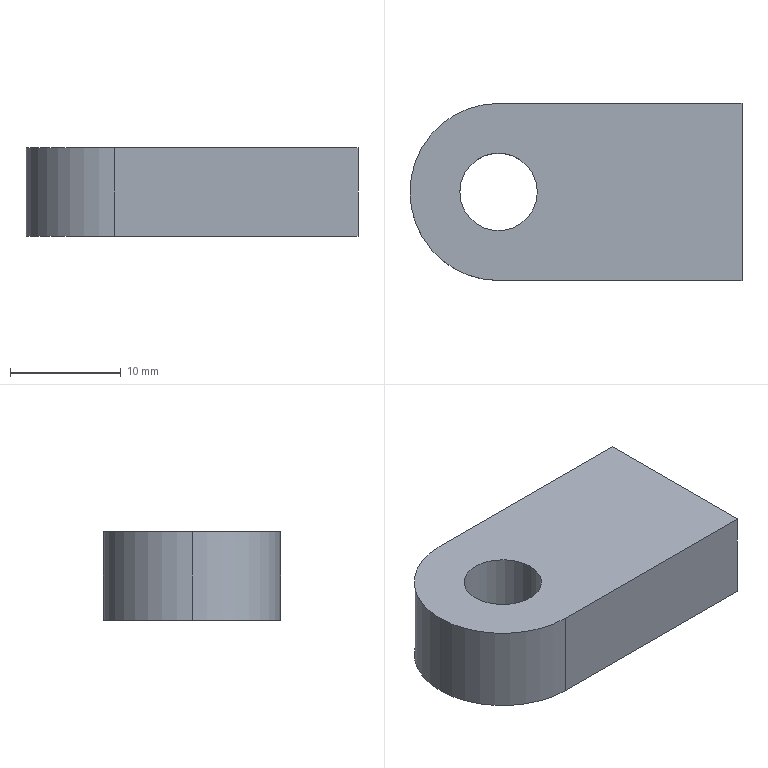Part | SolidWorks | features Extrusion 1 | 1 solid | 9 faces | box 30 x 16 x 8 mm | volume 3312 mm3 | plane 5 | cylinder 4 | commonest cylinder face diameters 7 x2 16 x2
STEP:
#1=CARTESIAN_POINT('',(-3.5,0.,8.));
#2=VERTEX_POINT('',#1);
#3=CARTESIAN_POINT('',(3.5,0.,8.));
#4=VERTEX_POINT('',#3);
#5=CARTESIAN_POINT('',(0.,0.,8.));
#6=DIRECTION('',(0.,0.,1.));
#7=DIRECTION('',(1.,0.,0.));
#8=AXIS2_PLACEMENT_3D('',#5,#6,#7);
#9=CIRCLE('',#8,3.5);
#10=EDGE_CURVE('',#2,#4,#9,.T.);
#11=ORIENTED_EDGE('',*,*,#10,.T.);
#12=CARTESIAN_POINT('',(3.5,0.,0.));
#13=VERTEX_POINT('',#12);
#14=CARTESIAN_POINT('',(3.5,0.,8.));
#15=DIRECTION('',(0.,0.,-1.));
#16=VECTOR('',#15,1000.);
#17=LINE('',#14,#16);
#18=EDGE_CURVE('',#4,#13,#17,.T.);
#19=ORIENTED_EDGE('',*,*,#18,.T.);
#20=CARTESIAN_POINT('',(-3.5,0.,0.));
#21=VERTEX_POINT('',#20);
#22=CARTESIAN_POINT('',(0.,0.,0.));
#23=DIRECTION('',(0.,0.,1.));
#24=DIRECTION('',(1.,0.,0.));
#25=AXIS2_PLACEMENT_3D('',#22,#23,#24);
#26=CIRCLE('',#25,3.5);
#27=EDGE_CURVE('',#21,#13,#26,.T.);
#28=ORIENTED_EDGE('',*,*,#27,.F.);
#29=CARTESIAN_POINT('',(-3.5,0.,8.));
#30=DIRECTION('',(0.,0.,-1.));
#31=VECTOR('',#30,1000.);
#32=LINE('',#29,#31);
#33=EDGE_CURVE('',#2,#21,#32,.T.);
#34=ORIENTED_EDGE('',*,*,#33,.F.);
#35=EDGE_LOOP('',(#11,#19,#28,#34));
#36=FACE_OUTER_BOUND('',#35,.T.);
#37=CARTESIAN_POINT('',(0.,0.,8.));
#38=DIRECTION('',(0.,0.,-1.));
#39=DIRECTION('',(-1.,0.,0.));
#40=AXIS2_PLACEMENT_3D('',#37,#38,#39);
#41=CYLINDRICAL_SURFACE('',#40,3.5);
#42=ADVANCED_FACE('',(#36),#41,.F.);
#43=CARTESIAN_POINT('',(-8.,0.,8.));
#44=VERTEX_POINT('',#43);
#45=CARTESIAN_POINT('',(0.,-8.,8.));
#46=VERTEX_POINT('',#45);
#47=CARTESIAN_POINT('',(0.,0.,8.));
#48=DIRECTION('',(0.,0.,1.));
#49=DIRECTION('',(1.,0.,0.));
#50=AXIS2_PLACEMENT_3D('',#47,#48,#49);
#51=CIRCLE('',#50,8.);
#52=EDGE_CURVE('',#44,#46,#51,.T.);
#53=ORIENTED_EDGE('',*,*,#52,.F.);
#54=CARTESIAN_POINT('',(-8.,0.,0.));
#55=VERTEX_POINT('',#54);
#56=CARTESIAN_POINT('',(-8.,0.,8.));
#57=DIRECTION('',(0.,0.,-1.));
#58=VECTOR('',#57,1000.);
#59=LINE('',#56,#58);
#60=EDGE_CURVE('',#44,#55,#59,.T.);
#61=ORIENTED_EDGE('',*,*,#60,.T.);
#62=CARTESIAN_POINT('',(0.,-8.,0.));
#63=VERTEX_POINT('',#62);
#64=CARTESIAN_POINT('',(0.,0.,0.));
#65=DIRECTION('',(0.,0.,1.));
#66=DIRECTION('',(1.,0.,0.));
#67=AXIS2_PLACEMENT_3D('',#64,#65,#66);
#68=CIRCLE('',#67,8.);
#69=EDGE_CURVE('',#55,#63,#68,.T.);
#70=ORIENTED_EDGE('',*,*,#69,.T.);
#71=CARTESIAN_POINT('',(0.,-8.,8.));
#72=DIRECTION('',(0.,0.,-1.));
#73=VECTOR('',#72,1000.);
#74=LINE('',#71,#73);
#75=EDGE_CURVE('',#46,#63,#74,.T.);
#76=ORIENTED_EDGE('',*,*,#75,.F.);
#77=EDGE_LOOP('',(#53,#61,#70,#76));
#78=FACE_OUTER_BOUND('',#77,.T.);
#79=CARTESIAN_POINT('',(0.,0.,8.));
#80=DIRECTION('',(0.,0.,-1.));
#81=DIRECTION('',(-1.,0.,0.));
#82=AXIS2_PLACEMENT_3D('',#79,#80,#81);
#83=CYLINDRICAL_SURFACE('',#82,8.);
#84=ADVANCED_FACE('',(#78),#83,.T.);
#85=CARTESIAN_POINT('',(0.,8.,8.));
#86=VERTEX_POINT('',#85);
#87=CARTESIAN_POINT('',(0.,0.,8.));
#88=DIRECTION('',(0.,0.,1.));
#89=DIRECTION('',(1.,0.,0.));
#90=AXIS2_PLACEMENT_3D('',#87,#88,#89);
#91=CIRCLE('',#90,8.);
#92=EDGE_CURVE('',#86,#44,#91,.T.);
#93=ORIENTED_EDGE('',*,*,#92,.T.);
#94=ORIENTED_EDGE('',*,*,#52,.T.);
#95=CARTESIAN_POINT('',(22.,-8.,8.));
#96=VERTEX_POINT('',#95);
#97=CARTESIAN_POINT('',(22.,-8.,8.));
#98=DIRECTION('',(1.,0.,0.));
#99=VECTOR('',#98,1000.);
#100=LINE('',#97,#99);
#101=EDGE_CURVE('',#46,#96,#100,.T.);
#102=ORIENTED_EDGE('',*,*,#101,.T.);
#103=CARTESIAN_POINT('',(22.,8.,8.));
#104=VERTEX_POINT('',#103);
#105=CARTESIAN_POINT('',(22.,8.,8.));
#106=DIRECTION('',(0.,1.,0.));
#107=VECTOR('',#106,1000.);
#108=LINE('',#105,#107);
#109=EDGE_CURVE('',#96,#104,#108,.T.);
#110=ORIENTED_EDGE('',*,*,#109,.T.);
#111=CARTESIAN_POINT('',(0.,8.,8.));
#112=DIRECTION('',(-1.,0.,0.));
#113=VECTOR('',#112,1000.);
#114=LINE('',#111,#113);
#115=EDGE_CURVE('',#104,#86,#114,.T.);
#116=ORIENTED_EDGE('',*,*,#115,.T.);
#117=EDGE_LOOP('',(#93,#94,#102,#110,#116));
#118=FACE_OUTER_BOUND('',#117,.T.);
#119=ORIENTED_EDGE('',*,*,#10,.F.);
#120=CARTESIAN_POINT('',(0.,0.,8.));
#121=DIRECTION('',(0.,0.,1.));
#122=DIRECTION('',(1.,0.,0.));
#123=AXIS2_PLACEMENT_3D('',#120,#121,#122);
#124=CIRCLE('',#123,3.5);
#125=EDGE_CURVE('',#4,#2,#124,.T.);
#126=ORIENTED_EDGE('',*,*,#125,.F.);
#127=EDGE_LOOP('',(#119,#126));
#128=FACE_BOUND('',#127,.T.);
#129=CARTESIAN_POINT('',(0.,0.,8.));
#130=DIRECTION('',(0.,0.,1.));
#131=DIRECTION('',(1.,0.,0.));
#132=AXIS2_PLACEMENT_3D('',#129,#130,#131);
#133=PLANE('',#132);
#134=ADVANCED_FACE('',(#118,#128),#133,.T.);
#135=CARTESIAN_POINT('',(0.,8.,0.));
#136=VERTEX_POINT('',#135);
#137=CARTESIAN_POINT('',(0.,0.,0.));
#138=DIRECTION('',(0.,0.,1.));
#139=DIRECTION('',(1.,0.,0.));
#140=AXIS2_PLACEMENT_3D('',#137,#138,#139);
#141=CIRCLE('',#140,8.);
#142=EDGE_CURVE('',#136,#55,#141,.T.);
#143=ORIENTED_EDGE('',*,*,#142,.F.);
#144=CARTESIAN_POINT('',(22.,8.,0.));
#145=VERTEX_POINT('',#144);
#146=CARTESIAN_POINT('',(0.,8.,0.));
#147=DIRECTION('',(-1.,0.,0.));
#148=VECTOR('',#147,1000.);
#149=LINE('',#146,#148);
#150=EDGE_CURVE('',#145,#136,#149,.T.);
#151=ORIENTED_EDGE('',*,*,#150,.F.);
#152=CARTESIAN_POINT('',(22.,-8.,0.));
#153=VERTEX_POINT('',#152);
#154=CARTESIAN_POINT('',(22.,8.,0.));
#155=DIRECTION('',(0.,1.,0.));
#156=VECTOR('',#155,1000.);
#157=LINE('',#154,#156);
#158=EDGE_CURVE('',#153,#145,#157,.T.);
#159=ORIENTED_EDGE('',*,*,#158,.F.);
#160=CARTESIAN_POINT('',(22.,-8.,0.));
#161=DIRECTION('',(1.,0.,0.));
#162=VECTOR('',#161,1000.);
#163=LINE('',#160,#162);
#164=EDGE_CURVE('',#63,#153,#163,.T.);
#165=ORIENTED_EDGE('',*,*,#164,.F.);
#166=ORIENTED_EDGE('',*,*,#69,.F.);
#167=EDGE_LOOP('',(#143,#151,#159,#165,#166));
#168=FACE_OUTER_BOUND('',#167,.T.);
#169=ORIENTED_EDGE('',*,*,#27,.T.);
#170=CARTESIAN_POINT('',(0.,0.,0.));
#171=DIRECTION('',(0.,0.,1.));
#172=DIRECTION('',(1.,0.,0.));
#173=AXIS2_PLACEMENT_3D('',#170,#171,#172);
#174=CIRCLE('',#173,3.5);
#175=EDGE_CURVE('',#13,#21,#174,.T.);
#176=ORIENTED_EDGE('',*,*,#175,.T.);
#177=EDGE_LOOP('',(#169,#176));
#178=FACE_BOUND('',#177,.T.);
#179=CARTESIAN_POINT('',(0.,0.,0.));
#180=DIRECTION('',(0.,0.,1.));
#181=DIRECTION('',(1.,0.,0.));
#182=AXIS2_PLACEMENT_3D('',#179,#180,#181);
#183=PLANE('',#182);
#184=ADVANCED_FACE('',(#168,#178),#183,.F.);
#185=ORIENTED_EDGE('',*,*,#60,.F.);
#186=ORIENTED_EDGE('',*,*,#92,.F.);
#187=CARTESIAN_POINT('',(0.,8.,8.));
#188=DIRECTION('',(0.,0.,-1.));
#189=VECTOR('',#188,1000.);
#190=LINE('',#187,#189);
#191=EDGE_CURVE('',#86,#136,#190,.T.);
#192=ORIENTED_EDGE('',*,*,#191,.T.);
#193=ORIENTED_EDGE('',*,*,#142,.T.);
#194=EDGE_LOOP('',(#185,#186,#192,#193));
#195=FACE_OUTER_BOUND('',#194,.T.);
#196=CARTESIAN_POINT('',(0.,0.,8.));
#197=DIRECTION('',(0.,0.,-1.));
#198=DIRECTION('',(-1.,0.,0.));
#199=AXIS2_PLACEMENT_3D('',#196,#197,#198);
#200=CYLINDRICAL_SURFACE('',#199,8.);
#201=ADVANCED_FACE('',(#195),#200,.T.);
#202=ORIENTED_EDGE('',*,*,#164,.T.);
#203=CARTESIAN_POINT('',(22.,-8.,8.));
#204=DIRECTION('',(0.,0.,-1.));
#205=VECTOR('',#204,1000.);
#206=LINE('',#203,#205);
#207=EDGE_CURVE('',#96,#153,#206,.T.);
#208=ORIENTED_EDGE('',*,*,#207,.F.);
#209=ORIENTED_EDGE('',*,*,#101,.F.);
#210=ORIENTED_EDGE('',*,*,#75,.T.);
#211=EDGE_LOOP('',(#202,#208,#209,#210));
#212=FACE_OUTER_BOUND('',#211,.T.);
#213=CARTESIAN_POINT('',(22.,-8.,8.));
#214=DIRECTION('',(0.,1.,0.));
#215=DIRECTION('',(-1.,0.,0.));
#216=AXIS2_PLACEMENT_3D('',#213,#214,#215);
#217=PLANE('',#216);
#218=ADVANCED_FACE('',(#212),#217,.F.);
#219=ORIENTED_EDGE('',*,*,#158,.T.);
#220=CARTESIAN_POINT('',(22.,8.,8.));
#221=DIRECTION('',(0.,0.,-1.));
#222=VECTOR('',#221,1000.);
#223=LINE('',#220,#222);
#224=EDGE_CURVE('',#104,#145,#223,.T.);
#225=ORIENTED_EDGE('',*,*,#224,.F.);
#226=ORIENTED_EDGE('',*,*,#109,.F.);
#227=ORIENTED_EDGE('',*,*,#207,.T.);
#228=EDGE_LOOP('',(#219,#225,#226,#227));
#229=FACE_OUTER_BOUND('',#228,.T.);
#230=CARTESIAN_POINT('',(22.,8.,8.));
#231=DIRECTION('',(-1.,0.,0.));
#232=DIRECTION('',(0.,0.,1.));
#233=AXIS2_PLACEMENT_3D('',#230,#231,#232);
#234=PLANE('',#233);
#235=ADVANCED_FACE('',(#229),#234,.F.);
#236=ORIENTED_EDGE('',*,*,#150,.T.);
#237=ORIENTED_EDGE('',*,*,#191,.F.);
#238=ORIENTED_EDGE('',*,*,#115,.F.);
#239=ORIENTED_EDGE('',*,*,#224,.T.);
#240=EDGE_LOOP('',(#236,#237,#238,#239));
#241=FACE_OUTER_BOUND('',#240,.T.);
#242=CARTESIAN_POINT('',(0.,8.,8.));
#243=DIRECTION('',(0.,-1.,0.));
#244=DIRECTION('',(1.,0.,0.));
#245=AXIS2_PLACEMENT_3D('',#242,#243,#244);
#246=PLANE('',#245);
#247=ADVANCED_FACE('',(#241),#246,.F.);
#248=ORIENTED_EDGE('',*,*,#18,.F.);
#249=ORIENTED_EDGE('',*,*,#125,.T.);
#250=ORIENTED_EDGE('',*,*,#33,.T.);
#251=ORIENTED_EDGE('',*,*,#175,.F.);
#252=EDGE_LOOP('',(#248,#249,#250,#251));
#253=FACE_OUTER_BOUND('',#252,.T.);
#254=CARTESIAN_POINT('',(0.,0.,8.));
#255=DIRECTION('',(0.,0.,-1.));
#256=DIRECTION('',(-1.,0.,0.));
#257=AXIS2_PLACEMENT_3D('',#254,#255,#256);
#258=CYLINDRICAL_SURFACE('',#257,3.5);
#259=ADVANCED_FACE('',(#253),#258,.F.);
#260=CLOSED_SHELL('',(#42,#84,#134,#184,#201,#218,#235,#247,#259));
#261=MANIFOLD_SOLID_BREP('',#260);
#262=CARTESIAN_POINT('',(0.,0.,0.));
#263=DIRECTION('',(0.,0.,1.));
#264=DIRECTION('',(1.,0.,0.));
#265=AXIS2_PLACEMENT_3D('',#262,#263,#264);
#266=(LENGTH_UNIT()NAMED_UNIT(*)SI_UNIT(.MILLI.,.METRE.));
#267=UNCERTAINTY_MEASURE_WITH_UNIT(LENGTH_MEASURE(0.00001),#266,'','');
#268=(NAMED_UNIT(*)PLANE_ANGLE_UNIT()SI_UNIT($,.RADIAN.));
#269=(NAMED_UNIT(*)SI_UNIT($,.STERADIAN.)SOLID_ANGLE_UNIT());
#270=(GEOMETRIC_REPRESENTATION_CONTEXT(3)GLOBAL_UNCERTAINTY_ASSIGNED_CONTEXT((#267))GLOBAL_UNIT_ASSIGNED_CONTEXT((#266,#268,#269))REPRESENTATION_CONTEXT('',''));
#271=ADVANCED_BREP_SHAPE_REPRESENTATION('',(#261,#265),#270);